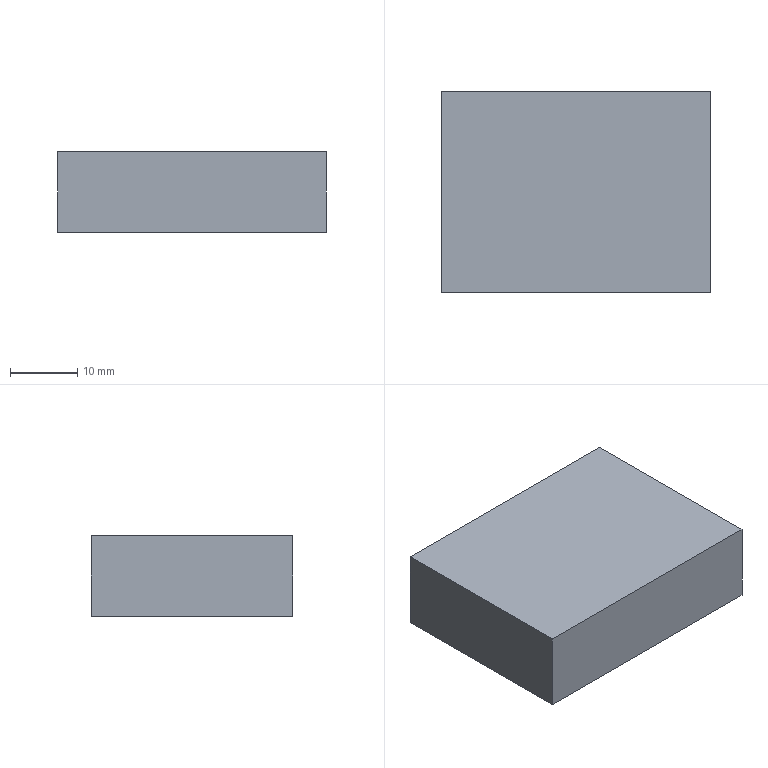Part | SolidWorks | features Extrusion 1 | 1 solid | 6 faces | box 40 x 30 x 12 mm | volume 14400 mm3 | plane 6
STEP:
#1=CARTESIAN_POINT('',(20.,-15.,-6.));
#2=VERTEX_POINT('',#1);
#3=CARTESIAN_POINT('',(20.,15.,-6.));
#4=VERTEX_POINT('',#3);
#5=CARTESIAN_POINT('',(20.,-15.,-6.));
#6=DIRECTION('',(0.,1.,0.));
#7=VECTOR('',#6,1000.);
#8=LINE('',#5,#7);
#9=EDGE_CURVE('',#2,#4,#8,.T.);
#10=ORIENTED_EDGE('',*,*,#9,.T.);
#11=CARTESIAN_POINT('',(20.,15.,6.));
#12=VERTEX_POINT('',#11);
#13=CARTESIAN_POINT('',(20.,15.,6.));
#14=DIRECTION('',(0.,0.,-1.));
#15=VECTOR('',#14,1000.);
#16=LINE('',#13,#15);
#17=EDGE_CURVE('',#12,#4,#16,.T.);
#18=ORIENTED_EDGE('',*,*,#17,.F.);
#19=CARTESIAN_POINT('',(20.,-15.,6.));
#20=VERTEX_POINT('',#19);
#21=CARTESIAN_POINT('',(20.,-15.,6.));
#22=DIRECTION('',(0.,1.,0.));
#23=VECTOR('',#22,1000.);
#24=LINE('',#21,#23);
#25=EDGE_CURVE('',#20,#12,#24,.T.);
#26=ORIENTED_EDGE('',*,*,#25,.F.);
#27=CARTESIAN_POINT('',(20.,-15.,6.));
#28=DIRECTION('',(0.,0.,-1.));
#29=VECTOR('',#28,1000.);
#30=LINE('',#27,#29);
#31=EDGE_CURVE('',#20,#2,#30,.T.);
#32=ORIENTED_EDGE('',*,*,#31,.T.);
#33=EDGE_LOOP('',(#10,#18,#26,#32));
#34=FACE_OUTER_BOUND('',#33,.T.);
#35=CARTESIAN_POINT('',(20.,-15.,6.));
#36=DIRECTION('',(-1.,0.,0.));
#37=DIRECTION('',(0.,0.,1.));
#38=AXIS2_PLACEMENT_3D('',#35,#36,#37);
#39=PLANE('',#38);
#40=ADVANCED_FACE('',(#34),#39,.F.);
#41=CARTESIAN_POINT('',(-20.,15.,-6.));
#42=VERTEX_POINT('',#41);
#43=CARTESIAN_POINT('',(-20.,15.,-6.));
#44=DIRECTION('',(-1.,0.,0.));
#45=VECTOR('',#44,1000.);
#46=LINE('',#43,#45);
#47=EDGE_CURVE('',#4,#42,#46,.T.);
#48=ORIENTED_EDGE('',*,*,#47,.T.);
#49=CARTESIAN_POINT('',(-20.,15.,6.));
#50=VERTEX_POINT('',#49);
#51=CARTESIAN_POINT('',(-20.,15.,6.));
#52=DIRECTION('',(0.,0.,-1.));
#53=VECTOR('',#52,1000.);
#54=LINE('',#51,#53);
#55=EDGE_CURVE('',#50,#42,#54,.T.);
#56=ORIENTED_EDGE('',*,*,#55,.F.);
#57=CARTESIAN_POINT('',(-20.,15.,6.));
#58=DIRECTION('',(-1.,0.,0.));
#59=VECTOR('',#58,1000.);
#60=LINE('',#57,#59);
#61=EDGE_CURVE('',#12,#50,#60,.T.);
#62=ORIENTED_EDGE('',*,*,#61,.F.);
#63=ORIENTED_EDGE('',*,*,#17,.T.);
#64=EDGE_LOOP('',(#48,#56,#62,#63));
#65=FACE_OUTER_BOUND('',#64,.T.);
#66=CARTESIAN_POINT('',(-20.,15.,6.));
#67=DIRECTION('',(0.,-1.,0.));
#68=DIRECTION('',(0.,0.,-1.));
#69=AXIS2_PLACEMENT_3D('',#66,#67,#68);
#70=PLANE('',#69);
#71=ADVANCED_FACE('',(#65),#70,.F.);
#72=CARTESIAN_POINT('',(-20.,-15.,-6.));
#73=VERTEX_POINT('',#72);
#74=CARTESIAN_POINT('',(-20.,-15.,-6.));
#75=DIRECTION('',(0.,-1.,0.));
#76=VECTOR('',#75,1000.);
#77=LINE('',#74,#76);
#78=EDGE_CURVE('',#42,#73,#77,.T.);
#79=ORIENTED_EDGE('',*,*,#78,.T.);
#80=CARTESIAN_POINT('',(-20.,-15.,6.));
#81=VERTEX_POINT('',#80);
#82=CARTESIAN_POINT('',(-20.,-15.,6.));
#83=DIRECTION('',(0.,0.,-1.));
#84=VECTOR('',#83,1000.);
#85=LINE('',#82,#84);
#86=EDGE_CURVE('',#81,#73,#85,.T.);
#87=ORIENTED_EDGE('',*,*,#86,.F.);
#88=CARTESIAN_POINT('',(-20.,-15.,6.));
#89=DIRECTION('',(0.,-1.,0.));
#90=VECTOR('',#89,1000.);
#91=LINE('',#88,#90);
#92=EDGE_CURVE('',#50,#81,#91,.T.);
#93=ORIENTED_EDGE('',*,*,#92,.F.);
#94=ORIENTED_EDGE('',*,*,#55,.T.);
#95=EDGE_LOOP('',(#79,#87,#93,#94));
#96=FACE_OUTER_BOUND('',#95,.T.);
#97=CARTESIAN_POINT('',(-20.,-15.,6.));
#98=DIRECTION('',(1.,0.,0.));
#99=DIRECTION('',(0.,0.,-1.));
#100=AXIS2_PLACEMENT_3D('',#97,#98,#99);
#101=PLANE('',#100);
#102=ADVANCED_FACE('',(#96),#101,.F.);
#103=CARTESIAN_POINT('',(-20.,-15.,-6.));
#104=DIRECTION('',(1.,0.,0.));
#105=VECTOR('',#104,1000.);
#106=LINE('',#103,#105);
#107=EDGE_CURVE('',#73,#2,#106,.T.);
#108=ORIENTED_EDGE('',*,*,#107,.T.);
#109=ORIENTED_EDGE('',*,*,#31,.F.);
#110=CARTESIAN_POINT('',(-20.,-15.,6.));
#111=DIRECTION('',(1.,0.,0.));
#112=VECTOR('',#111,1000.);
#113=LINE('',#110,#112);
#114=EDGE_CURVE('',#81,#20,#113,.T.);
#115=ORIENTED_EDGE('',*,*,#114,.F.);
#116=ORIENTED_EDGE('',*,*,#86,.T.);
#117=EDGE_LOOP('',(#108,#109,#115,#116));
#118=FACE_OUTER_BOUND('',#117,.T.);
#119=CARTESIAN_POINT('',(-20.,-15.,6.));
#120=DIRECTION('',(0.,1.,0.));
#121=DIRECTION('',(0.,0.,1.));
#122=AXIS2_PLACEMENT_3D('',#119,#120,#121);
#123=PLANE('',#122);
#124=ADVANCED_FACE('',(#118),#123,.F.);
#125=ORIENTED_EDGE('',*,*,#25,.T.);
#126=ORIENTED_EDGE('',*,*,#61,.T.);
#127=ORIENTED_EDGE('',*,*,#92,.T.);
#128=ORIENTED_EDGE('',*,*,#114,.T.);
#129=EDGE_LOOP('',(#125,#126,#127,#128));
#130=FACE_OUTER_BOUND('',#129,.T.);
#131=CARTESIAN_POINT('',(0.,0.,6.));
#132=DIRECTION('',(0.,0.,-1.));
#133=DIRECTION('',(-1.,0.,0.));
#134=AXIS2_PLACEMENT_3D('',#131,#132,#133);
#135=PLANE('',#134);
#136=ADVANCED_FACE('',(#130),#135,.F.);
#137=ORIENTED_EDGE('',*,*,#9,.F.);
#138=ORIENTED_EDGE('',*,*,#107,.F.);
#139=ORIENTED_EDGE('',*,*,#78,.F.);
#140=ORIENTED_EDGE('',*,*,#47,.F.);
#141=EDGE_LOOP('',(#137,#138,#139,#140));
#142=FACE_OUTER_BOUND('',#141,.T.);
#143=CARTESIAN_POINT('',(0.,0.,-6.));
#144=DIRECTION('',(0.,0.,-1.));
#145=DIRECTION('',(-1.,0.,0.));
#146=AXIS2_PLACEMENT_3D('',#143,#144,#145);
#147=PLANE('',#146);
#148=ADVANCED_FACE('',(#142),#147,.T.);
#149=CLOSED_SHELL('',(#40,#71,#102,#124,#136,#148));
#150=MANIFOLD_SOLID_BREP('',#149);
#151=CARTESIAN_POINT('',(0.,0.,0.));
#152=DIRECTION('',(0.,0.,1.));
#153=DIRECTION('',(1.,0.,0.));
#154=AXIS2_PLACEMENT_3D('',#151,#152,#153);
#155=(LENGTH_UNIT()NAMED_UNIT(*)SI_UNIT(.MILLI.,.METRE.));
#156=UNCERTAINTY_MEASURE_WITH_UNIT(LENGTH_MEASURE(0.00001),#155,'','');
#157=(NAMED_UNIT(*)PLANE_ANGLE_UNIT()SI_UNIT($,.RADIAN.));
#158=(NAMED_UNIT(*)SI_UNIT($,.STERADIAN.)SOLID_ANGLE_UNIT());
#159=(GEOMETRIC_REPRESENTATION_CONTEXT(3)GLOBAL_UNCERTAINTY_ASSIGNED_CONTEXT((#156))GLOBAL_UNIT_ASSIGNED_CONTEXT((#155,#157,#158))REPRESENTATION_CONTEXT('',''));
#160=ADVANCED_BREP_SHAPE_REPRESENTATION('',(#150,#154),#159);